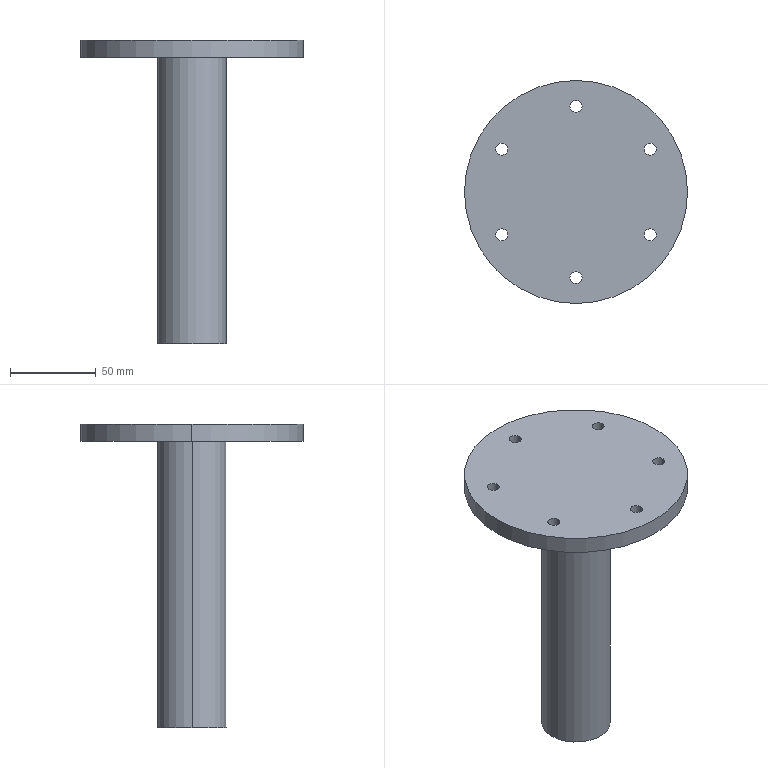Part | SolidWorks | features BaseBody 1 | 1 solid | 22 faces | box 130 x 130 x 177.2 mm | volume 222346 mm3 | cylinder 18 | plane 4 | commonest cylinder face diameters 7 x12 30 x2 40 x2 130 x2
STEP:
#1=CARTESIAN_POINT('',(39.801,25.,167.2));
#2=VERTEX_POINT('',#1);
#3=CARTESIAN_POINT('',(46.801,25.,167.2));
#4=VERTEX_POINT('',#3);
#5=CARTESIAN_POINT('',(43.301,25.,167.2));
#6=DIRECTION('',(0.,0.,1.));
#7=DIRECTION('',(1.,0.,0.));
#8=AXIS2_PLACEMENT_3D('',#5,#6,#7);
#9=CIRCLE('',#8,3.5);
#10=EDGE_CURVE('',#2,#4,#9,.T.);
#11=ORIENTED_EDGE('',*,*,#10,.F.);
#12=CARTESIAN_POINT('',(39.801,25.,177.2));
#13=VERTEX_POINT('',#12);
#14=CARTESIAN_POINT('',(39.801,25.,167.2));
#15=DIRECTION('',(0.,0.,1.));
#16=VECTOR('',#15,1000.);
#17=LINE('',#14,#16);
#18=EDGE_CURVE('',#2,#13,#17,.T.);
#19=ORIENTED_EDGE('',*,*,#18,.T.);
#20=CARTESIAN_POINT('',(46.801,25.,177.2));
#21=VERTEX_POINT('',#20);
#22=CARTESIAN_POINT('',(43.301,25.,177.2));
#23=DIRECTION('',(0.,0.,1.));
#24=DIRECTION('',(1.,0.,0.));
#25=AXIS2_PLACEMENT_3D('',#22,#23,#24);
#26=CIRCLE('',#25,3.5);
#27=EDGE_CURVE('',#13,#21,#26,.T.);
#28=ORIENTED_EDGE('',*,*,#27,.T.);
#29=CARTESIAN_POINT('',(46.801,25.,167.2));
#30=DIRECTION('',(0.,0.,1.));
#31=VECTOR('',#30,1000.);
#32=LINE('',#29,#31);
#33=EDGE_CURVE('',#4,#21,#32,.T.);
#34=ORIENTED_EDGE('',*,*,#33,.F.);
#35=EDGE_LOOP('',(#11,#19,#28,#34));
#36=FACE_OUTER_BOUND('',#35,.T.);
#37=CARTESIAN_POINT('',(43.301,25.,167.2));
#38=DIRECTION('',(0.,0.,1.));
#39=DIRECTION('',(1.,0.,0.));
#40=AXIS2_PLACEMENT_3D('',#37,#38,#39);
#41=CYLINDRICAL_SURFACE('',#40,3.5);
#42=ADVANCED_FACE('',(#36),#41,.F.);
#43=CARTESIAN_POINT('',(39.801,-25.,167.2));
#44=VERTEX_POINT('',#43);
#45=CARTESIAN_POINT('',(46.801,-25.,167.2));
#46=VERTEX_POINT('',#45);
#47=CARTESIAN_POINT('',(43.301,-25.,167.2));
#48=DIRECTION('',(0.,0.,1.));
#49=DIRECTION('',(1.,0.,0.));
#50=AXIS2_PLACEMENT_3D('',#47,#48,#49);
#51=CIRCLE('',#50,3.5);
#52=EDGE_CURVE('',#44,#46,#51,.T.);
#53=ORIENTED_EDGE('',*,*,#52,.F.);
#54=CARTESIAN_POINT('',(39.801,-25.,177.2));
#55=VERTEX_POINT('',#54);
#56=CARTESIAN_POINT('',(39.801,-25.,167.2));
#57=DIRECTION('',(0.,0.,1.));
#58=VECTOR('',#57,1000.);
#59=LINE('',#56,#58);
#60=EDGE_CURVE('',#44,#55,#59,.T.);
#61=ORIENTED_EDGE('',*,*,#60,.T.);
#62=CARTESIAN_POINT('',(46.801,-25.,177.2));
#63=VERTEX_POINT('',#62);
#64=CARTESIAN_POINT('',(43.301,-25.,177.2));
#65=DIRECTION('',(0.,0.,1.));
#66=DIRECTION('',(1.,0.,0.));
#67=AXIS2_PLACEMENT_3D('',#64,#65,#66);
#68=CIRCLE('',#67,3.5);
#69=EDGE_CURVE('',#55,#63,#68,.T.);
#70=ORIENTED_EDGE('',*,*,#69,.T.);
#71=CARTESIAN_POINT('',(46.801,-25.,167.2));
#72=DIRECTION('',(0.,0.,1.));
#73=VECTOR('',#72,1000.);
#74=LINE('',#71,#73);
#75=EDGE_CURVE('',#46,#63,#74,.T.);
#76=ORIENTED_EDGE('',*,*,#75,.F.);
#77=EDGE_LOOP('',(#53,#61,#70,#76));
#78=FACE_OUTER_BOUND('',#77,.T.);
#79=CARTESIAN_POINT('',(43.301,-25.,167.2));
#80=DIRECTION('',(0.,0.,1.));
#81=DIRECTION('',(1.,0.,0.));
#82=AXIS2_PLACEMENT_3D('',#79,#80,#81);
#83=CYLINDRICAL_SURFACE('',#82,3.5);
#84=ADVANCED_FACE('',(#78),#83,.F.);
#85=CARTESIAN_POINT('',(-3.5,-50.,167.2));
#86=VERTEX_POINT('',#85);
#87=CARTESIAN_POINT('',(3.5,-50.,167.2));
#88=VERTEX_POINT('',#87);
#89=CARTESIAN_POINT('',(0.,-50.,167.2));
#90=DIRECTION('',(0.,0.,1.));
#91=DIRECTION('',(1.,0.,0.));
#92=AXIS2_PLACEMENT_3D('',#89,#90,#91);
#93=CIRCLE('',#92,3.5);
#94=EDGE_CURVE('',#86,#88,#93,.T.);
#95=ORIENTED_EDGE('',*,*,#94,.F.);
#96=CARTESIAN_POINT('',(-3.5,-50.,177.2));
#97=VERTEX_POINT('',#96);
#98=CARTESIAN_POINT('',(-3.5,-50.,167.2));
#99=DIRECTION('',(0.,0.,1.));
#100=VECTOR('',#99,1000.);
#101=LINE('',#98,#100);
#102=EDGE_CURVE('',#86,#97,#101,.T.);
#103=ORIENTED_EDGE('',*,*,#102,.T.);
#104=CARTESIAN_POINT('',(3.5,-50.,177.2));
#105=VERTEX_POINT('',#104);
#106=CARTESIAN_POINT('',(0.,-50.,177.2));
#107=DIRECTION('',(0.,0.,1.));
#108=DIRECTION('',(1.,0.,0.));
#109=AXIS2_PLACEMENT_3D('',#106,#107,#108);
#110=CIRCLE('',#109,3.5);
#111=EDGE_CURVE('',#97,#105,#110,.T.);
#112=ORIENTED_EDGE('',*,*,#111,.T.);
#113=CARTESIAN_POINT('',(3.5,-50.,167.2));
#114=DIRECTION('',(0.,0.,1.));
#115=VECTOR('',#114,1000.);
#116=LINE('',#113,#115);
#117=EDGE_CURVE('',#88,#105,#116,.T.);
#118=ORIENTED_EDGE('',*,*,#117,.F.);
#119=EDGE_LOOP('',(#95,#103,#112,#118));
#120=FACE_OUTER_BOUND('',#119,.T.);
#121=CARTESIAN_POINT('',(0.,-50.,167.2));
#122=DIRECTION('',(0.,0.,1.));
#123=DIRECTION('',(1.,0.,0.));
#124=AXIS2_PLACEMENT_3D('',#121,#122,#123);
#125=CYLINDRICAL_SURFACE('',#124,3.5);
#126=ADVANCED_FACE('',(#120),#125,.F.);
#127=CARTESIAN_POINT('',(-46.801,-25.,167.2));
#128=VERTEX_POINT('',#127);
#129=CARTESIAN_POINT('',(-39.801,-25.,167.2));
#130=VERTEX_POINT('',#129);
#131=CARTESIAN_POINT('',(-43.301,-25.,167.2));
#132=DIRECTION('',(0.,0.,1.));
#133=DIRECTION('',(1.,0.,0.));
#134=AXIS2_PLACEMENT_3D('',#131,#132,#133);
#135=CIRCLE('',#134,3.5);
#136=EDGE_CURVE('',#128,#130,#135,.T.);
#137=ORIENTED_EDGE('',*,*,#136,.F.);
#138=CARTESIAN_POINT('',(-46.801,-25.,177.2));
#139=VERTEX_POINT('',#138);
#140=CARTESIAN_POINT('',(-46.801,-25.,167.2));
#141=DIRECTION('',(0.,0.,1.));
#142=VECTOR('',#141,1000.);
#143=LINE('',#140,#142);
#144=EDGE_CURVE('',#128,#139,#143,.T.);
#145=ORIENTED_EDGE('',*,*,#144,.T.);
#146=CARTESIAN_POINT('',(-39.801,-25.,177.2));
#147=VERTEX_POINT('',#146);
#148=CARTESIAN_POINT('',(-43.301,-25.,177.2));
#149=DIRECTION('',(0.,0.,1.));
#150=DIRECTION('',(1.,0.,0.));
#151=AXIS2_PLACEMENT_3D('',#148,#149,#150);
#152=CIRCLE('',#151,3.5);
#153=EDGE_CURVE('',#139,#147,#152,.T.);
#154=ORIENTED_EDGE('',*,*,#153,.T.);
#155=CARTESIAN_POINT('',(-39.801,-25.,167.2));
#156=DIRECTION('',(0.,0.,1.));
#157=VECTOR('',#156,1000.);
#158=LINE('',#155,#157);
#159=EDGE_CURVE('',#130,#147,#158,.T.);
#160=ORIENTED_EDGE('',*,*,#159,.F.);
#161=EDGE_LOOP('',(#137,#145,#154,#160));
#162=FACE_OUTER_BOUND('',#161,.T.);
#163=CARTESIAN_POINT('',(-43.301,-25.,167.2));
#164=DIRECTION('',(0.,0.,1.));
#165=DIRECTION('',(1.,0.,0.));
#166=AXIS2_PLACEMENT_3D('',#163,#164,#165);
#167=CYLINDRICAL_SURFACE('',#166,3.5);
#168=ADVANCED_FACE('',(#162),#167,.F.);
#169=CARTESIAN_POINT('',(-46.801,25.,167.2));
#170=VERTEX_POINT('',#169);
#171=CARTESIAN_POINT('',(-39.801,25.,167.2));
#172=VERTEX_POINT('',#171);
#173=CARTESIAN_POINT('',(-43.301,25.,167.2));
#174=DIRECTION('',(0.,0.,1.));
#175=DIRECTION('',(1.,0.,0.));
#176=AXIS2_PLACEMENT_3D('',#173,#174,#175);
#177=CIRCLE('',#176,3.5);
#178=EDGE_CURVE('',#170,#172,#177,.T.);
#179=ORIENTED_EDGE('',*,*,#178,.F.);
#180=CARTESIAN_POINT('',(-46.801,25.,177.2));
#181=VERTEX_POINT('',#180);
#182=CARTESIAN_POINT('',(-46.801,25.,167.2));
#183=DIRECTION('',(0.,0.,1.));
#184=VECTOR('',#183,1000.);
#185=LINE('',#182,#184);
#186=EDGE_CURVE('',#170,#181,#185,.T.);
#187=ORIENTED_EDGE('',*,*,#186,.T.);
#188=CARTESIAN_POINT('',(-39.801,25.,177.2));
#189=VERTEX_POINT('',#188);
#190=CARTESIAN_POINT('',(-43.301,25.,177.2));
#191=DIRECTION('',(0.,0.,1.));
#192=DIRECTION('',(1.,0.,0.));
#193=AXIS2_PLACEMENT_3D('',#190,#191,#192);
#194=CIRCLE('',#193,3.5);
#195=EDGE_CURVE('',#181,#189,#194,.T.);
#196=ORIENTED_EDGE('',*,*,#195,.T.);
#197=CARTESIAN_POINT('',(-39.801,25.,167.2));
#198=DIRECTION('',(0.,0.,1.));
#199=VECTOR('',#198,1000.);
#200=LINE('',#197,#199);
#201=EDGE_CURVE('',#172,#189,#200,.T.);
#202=ORIENTED_EDGE('',*,*,#201,.F.);
#203=EDGE_LOOP('',(#179,#187,#196,#202));
#204=FACE_OUTER_BOUND('',#203,.T.);
#205=CARTESIAN_POINT('',(-43.301,25.,167.2));
#206=DIRECTION('',(0.,0.,1.));
#207=DIRECTION('',(1.,0.,0.));
#208=AXIS2_PLACEMENT_3D('',#205,#206,#207);
#209=CYLINDRICAL_SURFACE('',#208,3.5);
#210=ADVANCED_FACE('',(#204),#209,.F.);
#211=CARTESIAN_POINT('',(-3.5,50.,167.2));
#212=VERTEX_POINT('',#211);
#213=CARTESIAN_POINT('',(3.5,50.,167.2));
#214=VERTEX_POINT('',#213);
#215=CARTESIAN_POINT('',(0.,50.,167.2));
#216=DIRECTION('',(0.,0.,1.));
#217=DIRECTION('',(1.,0.,0.));
#218=AXIS2_PLACEMENT_3D('',#215,#216,#217);
#219=CIRCLE('',#218,3.5);
#220=EDGE_CURVE('',#212,#214,#219,.T.);
#221=ORIENTED_EDGE('',*,*,#220,.F.);
#222=CARTESIAN_POINT('',(-3.5,50.,177.2));
#223=VERTEX_POINT('',#222);
#224=CARTESIAN_POINT('',(-3.5,50.,167.2));
#225=DIRECTION('',(0.,0.,1.));
#226=VECTOR('',#225,1000.);
#227=LINE('',#224,#226);
#228=EDGE_CURVE('',#212,#223,#227,.T.);
#229=ORIENTED_EDGE('',*,*,#228,.T.);
#230=CARTESIAN_POINT('',(3.5,50.,177.2));
#231=VERTEX_POINT('',#230);
#232=CARTESIAN_POINT('',(0.,50.,177.2));
#233=DIRECTION('',(0.,0.,1.));
#234=DIRECTION('',(1.,0.,0.));
#235=AXIS2_PLACEMENT_3D('',#232,#233,#234);
#236=CIRCLE('',#235,3.5);
#237=EDGE_CURVE('',#223,#231,#236,.T.);
#238=ORIENTED_EDGE('',*,*,#237,.T.);
#239=CARTESIAN_POINT('',(3.5,50.,167.2));
#240=DIRECTION('',(0.,0.,1.));
#241=VECTOR('',#240,1000.);
#242=LINE('',#239,#241);
#243=EDGE_CURVE('',#214,#231,#242,.T.);
#244=ORIENTED_EDGE('',*,*,#243,.F.);
#245=EDGE_LOOP('',(#221,#229,#238,#244));
#246=FACE_OUTER_BOUND('',#245,.T.);
#247=CARTESIAN_POINT('',(0.,50.,167.2));
#248=DIRECTION('',(0.,0.,1.));
#249=DIRECTION('',(1.,0.,0.));
#250=AXIS2_PLACEMENT_3D('',#247,#248,#249);
#251=CYLINDRICAL_SURFACE('',#250,3.5);
#252=ADVANCED_FACE('',(#246),#251,.F.);
#253=CARTESIAN_POINT('',(65.,0.,167.2));
#254=VERTEX_POINT('',#253);
#255=CARTESIAN_POINT('',(-65.,0.,167.2));
#256=VERTEX_POINT('',#255);
#257=CARTESIAN_POINT('',(0.,0.,167.2));
#258=DIRECTION('',(0.,0.,1.));
#259=DIRECTION('',(1.,0.,0.));
#260=AXIS2_PLACEMENT_3D('',#257,#258,#259);
#261=CIRCLE('',#260,65.);
#262=EDGE_CURVE('',#254,#256,#261,.T.);
#263=ORIENTED_EDGE('',*,*,#262,.T.);
#264=CARTESIAN_POINT('',(-65.,0.,177.2));
#265=VERTEX_POINT('',#264);
#266=CARTESIAN_POINT('',(-65.,0.,167.2));
#267=DIRECTION('',(0.,0.,1.));
#268=VECTOR('',#267,1000.);
#269=LINE('',#266,#268);
#270=EDGE_CURVE('',#256,#265,#269,.T.);
#271=ORIENTED_EDGE('',*,*,#270,.T.);
#272=CARTESIAN_POINT('',(65.,0.,177.2));
#273=VERTEX_POINT('',#272);
#274=CARTESIAN_POINT('',(0.,0.,177.2));
#275=DIRECTION('',(0.,0.,-1.));
#276=DIRECTION('',(1.,0.,0.));
#277=AXIS2_PLACEMENT_3D('',#274,#275,#276);
#278=CIRCLE('',#277,65.);
#279=EDGE_CURVE('',#265,#273,#278,.T.);
#280=ORIENTED_EDGE('',*,*,#279,.T.);
#281=CARTESIAN_POINT('',(65.,0.,167.2));
#282=DIRECTION('',(0.,0.,1.));
#283=VECTOR('',#282,1000.);
#284=LINE('',#281,#283);
#285=EDGE_CURVE('',#254,#273,#284,.T.);
#286=ORIENTED_EDGE('',*,*,#285,.F.);
#287=EDGE_LOOP('',(#263,#271,#280,#286));
#288=FACE_OUTER_BOUND('',#287,.T.);
#289=CARTESIAN_POINT('',(0.,0.,167.2));
#290=DIRECTION('',(0.,0.,1.));
#291=DIRECTION('',(1.,0.,0.));
#292=AXIS2_PLACEMENT_3D('',#289,#290,#291);
#293=CYLINDRICAL_SURFACE('',#292,65.);
#294=ADVANCED_FACE('',(#288),#293,.T.);
#295=CARTESIAN_POINT('',(20.,0.,167.2));
#296=VERTEX_POINT('',#295);
#297=CARTESIAN_POINT('',(-20.,0.,167.2));
#298=VERTEX_POINT('',#297);
#299=CARTESIAN_POINT('',(0.,0.,167.2));
#300=DIRECTION('',(0.,0.,1.));
#301=DIRECTION('',(-1.,0.,0.));
#302=AXIS2_PLACEMENT_3D('',#299,#300,#301);
#303=CIRCLE('',#302,20.);
#304=EDGE_CURVE('',#296,#298,#303,.T.);
#305=ORIENTED_EDGE('',*,*,#304,.F.);
#306=CARTESIAN_POINT('',(20.,0.,0.));
#307=VERTEX_POINT('',#306);
#308=CARTESIAN_POINT('',(20.,0.,233.769));
#309=DIRECTION('',(0.,0.,-1.));
#310=VECTOR('',#309,1000.);
#311=LINE('',#308,#310);
#312=EDGE_CURVE('',#296,#307,#311,.T.);
#313=ORIENTED_EDGE('',*,*,#312,.T.);
#314=CARTESIAN_POINT('',(-20.,0.,0.));
#315=VERTEX_POINT('',#314);
#316=CARTESIAN_POINT('',(0.,0.,0.));
#317=DIRECTION('',(0.,0.,1.));
#318=DIRECTION('',(-1.,0.,0.));
#319=AXIS2_PLACEMENT_3D('',#316,#317,#318);
#320=CIRCLE('',#319,20.);
#321=EDGE_CURVE('',#307,#315,#320,.T.);
#322=ORIENTED_EDGE('',*,*,#321,.T.);
#323=CARTESIAN_POINT('',(-20.,0.,233.769));
#324=DIRECTION('',(0.,0.,-1.));
#325=VECTOR('',#324,1000.);
#326=LINE('',#323,#325);
#327=EDGE_CURVE('',#298,#315,#326,.T.);
#328=ORIENTED_EDGE('',*,*,#327,.F.);
#329=EDGE_LOOP('',(#305,#313,#322,#328));
#330=FACE_OUTER_BOUND('',#329,.T.);
#331=CARTESIAN_POINT('',(0.,0.,233.769));
#332=DIRECTION('',(0.,0.,-1.));
#333=DIRECTION('',(-1.,0.,0.));
#334=AXIS2_PLACEMENT_3D('',#331,#332,#333);
#335=CYLINDRICAL_SURFACE('',#334,20.);
#336=ADVANCED_FACE('',(#330),#335,.T.);
#337=CARTESIAN_POINT('',(15.,0.,167.2));
#338=VERTEX_POINT('',#337);
#339=CARTESIAN_POINT('',(-15.,0.,167.2));
#340=VERTEX_POINT('',#339);
#341=CARTESIAN_POINT('',(0.,0.,167.2));
#342=DIRECTION('',(0.,0.,-1.));
#343=DIRECTION('',(-1.,0.,0.));
#344=AXIS2_PLACEMENT_3D('',#341,#342,#343);
#345=CIRCLE('',#344,15.);
#346=EDGE_CURVE('',#338,#340,#345,.T.);
#347=ORIENTED_EDGE('',*,*,#346,.F.);
#348=CARTESIAN_POINT('',(15.,0.,0.));
#349=VERTEX_POINT('',#348);
#350=CARTESIAN_POINT('',(15.,0.,233.769));
#351=DIRECTION('',(0.,0.,-1.));
#352=VECTOR('',#351,1000.);
#353=LINE('',#350,#352);
#354=EDGE_CURVE('',#338,#349,#353,.T.);
#355=ORIENTED_EDGE('',*,*,#354,.T.);
#356=CARTESIAN_POINT('',(-15.,0.,0.));
#357=VERTEX_POINT('',#356);
#358=CARTESIAN_POINT('',(0.,0.,0.));
#359=DIRECTION('',(0.,0.,-1.));
#360=DIRECTION('',(-1.,0.,0.));
#361=AXIS2_PLACEMENT_3D('',#358,#359,#360);
#362=CIRCLE('',#361,15.);
#363=EDGE_CURVE('',#349,#357,#362,.T.);
#364=ORIENTED_EDGE('',*,*,#363,.T.);
#365=CARTESIAN_POINT('',(-15.,0.,233.769));
#366=DIRECTION('',(0.,0.,-1.));
#367=VECTOR('',#366,1000.);
#368=LINE('',#365,#367);
#369=EDGE_CURVE('',#340,#357,#368,.T.);
#370=ORIENTED_EDGE('',*,*,#369,.F.);
#371=EDGE_LOOP('',(#347,#355,#364,#370));
#372=FACE_OUTER_BOUND('',#371,.T.);
#373=CARTESIAN_POINT('',(0.,0.,233.769));
#374=DIRECTION('',(0.,0.,-1.));
#375=DIRECTION('',(-1.,0.,0.));
#376=AXIS2_PLACEMENT_3D('',#373,#374,#375);
#377=CYLINDRICAL_SURFACE('',#376,15.);
#378=ADVANCED_FACE('',(#372),#377,.F.);
#379=CARTESIAN_POINT('',(43.301,25.,177.2));
#380=DIRECTION('',(0.,0.,1.));
#381=DIRECTION('',(1.,0.,0.));
#382=AXIS2_PLACEMENT_3D('',#379,#380,#381);
#383=CIRCLE('',#382,3.5);
#384=EDGE_CURVE('',#21,#13,#383,.T.);
#385=ORIENTED_EDGE('',*,*,#384,.F.);
#386=ORIENTED_EDGE('',*,*,#27,.F.);
#387=EDGE_LOOP('',(#385,#386));
#388=FACE_BOUND('',#387,.T.);
#389=CARTESIAN_POINT('',(43.301,-25.,177.2));
#390=DIRECTION('',(0.,0.,1.));
#391=DIRECTION('',(1.,0.,0.));
#392=AXIS2_PLACEMENT_3D('',#389,#390,#391);
#393=CIRCLE('',#392,3.5);
#394=EDGE_CURVE('',#63,#55,#393,.T.);
#395=ORIENTED_EDGE('',*,*,#394,.F.);
#396=ORIENTED_EDGE('',*,*,#69,.F.);
#397=EDGE_LOOP('',(#395,#396));
#398=FACE_BOUND('',#397,.T.);
#399=CARTESIAN_POINT('',(0.,-50.,177.2));
#400=DIRECTION('',(0.,0.,1.));
#401=DIRECTION('',(1.,0.,0.));
#402=AXIS2_PLACEMENT_3D('',#399,#400,#401);
#403=CIRCLE('',#402,3.5);
#404=EDGE_CURVE('',#105,#97,#403,.T.);
#405=ORIENTED_EDGE('',*,*,#404,.F.);
#406=ORIENTED_EDGE('',*,*,#111,.F.);
#407=EDGE_LOOP('',(#405,#406));
#408=FACE_BOUND('',#407,.T.);
#409=CARTESIAN_POINT('',(-43.301,-25.,177.2));
#410=DIRECTION('',(0.,0.,1.));
#411=DIRECTION('',(1.,0.,0.));
#412=AXIS2_PLACEMENT_3D('',#409,#410,#411);
#413=CIRCLE('',#412,3.5);
#414=EDGE_CURVE('',#147,#139,#413,.T.);
#415=ORIENTED_EDGE('',*,*,#414,.F.);
#416=ORIENTED_EDGE('',*,*,#153,.F.);
#417=EDGE_LOOP('',(#415,#416));
#418=FACE_BOUND('',#417,.T.);
#419=CARTESIAN_POINT('',(-43.301,25.,177.2));
#420=DIRECTION('',(0.,0.,1.));
#421=DIRECTION('',(1.,0.,0.));
#422=AXIS2_PLACEMENT_3D('',#419,#420,#421);
#423=CIRCLE('',#422,3.5);
#424=EDGE_CURVE('',#189,#181,#423,.T.);
#425=ORIENTED_EDGE('',*,*,#424,.F.);
#426=ORIENTED_EDGE('',*,*,#195,.F.);
#427=EDGE_LOOP('',(#425,#426));
#428=FACE_BOUND('',#427,.T.);
#429=CARTESIAN_POINT('',(0.,50.,177.2));
#430=DIRECTION('',(0.,0.,1.));
#431=DIRECTION('',(1.,0.,0.));
#432=AXIS2_PLACEMENT_3D('',#429,#430,#431);
#433=CIRCLE('',#432,3.5);
#434=EDGE_CURVE('',#231,#223,#433,.T.);
#435=ORIENTED_EDGE('',*,*,#434,.F.);
#436=ORIENTED_EDGE('',*,*,#237,.F.);
#437=EDGE_LOOP('',(#435,#436));
#438=FACE_BOUND('',#437,.T.);
#439=CARTESIAN_POINT('',(0.,0.,177.2));
#440=DIRECTION('',(0.,0.,-1.));
#441=DIRECTION('',(1.,0.,0.));
#442=AXIS2_PLACEMENT_3D('',#439,#440,#441);
#443=CIRCLE('',#442,65.);
#444=EDGE_CURVE('',#273,#265,#443,.T.);
#445=ORIENTED_EDGE('',*,*,#444,.F.);
#446=ORIENTED_EDGE('',*,*,#279,.F.);
#447=EDGE_LOOP('',(#445,#446));
#448=FACE_OUTER_BOUND('',#447,.T.);
#449=CARTESIAN_POINT('',(431.187,336.743,177.2));
#450=DIRECTION('',(0.,0.,-1.));
#451=DIRECTION('',(0.,1.,0.));
#452=AXIS2_PLACEMENT_3D('',#449,#450,#451);
#453=PLANE('',#452);
#454=ADVANCED_FACE('',(#388,#398,#408,#418,#428,#438,#448),#453,.F.);
#455=ORIENTED_EDGE('',*,*,#18,.F.);
#456=CARTESIAN_POINT('',(43.301,25.,167.2));
#457=DIRECTION('',(0.,0.,1.));
#458=DIRECTION('',(1.,0.,0.));
#459=AXIS2_PLACEMENT_3D('',#456,#457,#458);
#460=CIRCLE('',#459,3.5);
#461=EDGE_CURVE('',#4,#2,#460,.T.);
#462=ORIENTED_EDGE('',*,*,#461,.F.);
#463=ORIENTED_EDGE('',*,*,#33,.T.);
#464=ORIENTED_EDGE('',*,*,#384,.T.);
#465=EDGE_LOOP('',(#455,#462,#463,#464));
#466=FACE_OUTER_BOUND('',#465,.T.);
#467=CARTESIAN_POINT('',(43.301,25.,167.2));
#468=DIRECTION('',(0.,0.,1.));
#469=DIRECTION('',(1.,0.,0.));
#470=AXIS2_PLACEMENT_3D('',#467,#468,#469);
#471=CYLINDRICAL_SURFACE('',#470,3.5);
#472=ADVANCED_FACE('',(#466),#471,.F.);
#473=ORIENTED_EDGE('',*,*,#60,.F.);
#474=CARTESIAN_POINT('',(43.301,-25.,167.2));
#475=DIRECTION('',(0.,0.,1.));
#476=DIRECTION('',(1.,0.,0.));
#477=AXIS2_PLACEMENT_3D('',#474,#475,#476);
#478=CIRCLE('',#477,3.5);
#479=EDGE_CURVE('',#46,#44,#478,.T.);
#480=ORIENTED_EDGE('',*,*,#479,.F.);
#481=ORIENTED_EDGE('',*,*,#75,.T.);
#482=ORIENTED_EDGE('',*,*,#394,.T.);
#483=EDGE_LOOP('',(#473,#480,#481,#482));
#484=FACE_OUTER_BOUND('',#483,.T.);
#485=CARTESIAN_POINT('',(43.301,-25.,167.2));
#486=DIRECTION('',(0.,0.,1.));
#487=DIRECTION('',(1.,0.,0.));
#488=AXIS2_PLACEMENT_3D('',#485,#486,#487);
#489=CYLINDRICAL_SURFACE('',#488,3.5);
#490=ADVANCED_FACE('',(#484),#489,.F.);
#491=ORIENTED_EDGE('',*,*,#102,.F.);
#492=CARTESIAN_POINT('',(0.,-50.,167.2));
#493=DIRECTION('',(0.,0.,1.));
#494=DIRECTION('',(1.,0.,0.));
#495=AXIS2_PLACEMENT_3D('',#492,#493,#494);
#496=CIRCLE('',#495,3.5);
#497=EDGE_CURVE('',#88,#86,#496,.T.);
#498=ORIENTED_EDGE('',*,*,#497,.F.);
#499=ORIENTED_EDGE('',*,*,#117,.T.);
#500=ORIENTED_EDGE('',*,*,#404,.T.);
#501=EDGE_LOOP('',(#491,#498,#499,#500));
#502=FACE_OUTER_BOUND('',#501,.T.);
#503=CARTESIAN_POINT('',(0.,-50.,167.2));
#504=DIRECTION('',(0.,0.,1.));
#505=DIRECTION('',(1.,0.,0.));
#506=AXIS2_PLACEMENT_3D('',#503,#504,#505);
#507=CYLINDRICAL_SURFACE('',#506,3.5);
#508=ADVANCED_FACE('',(#502),#507,.F.);
#509=ORIENTED_EDGE('',*,*,#144,.F.);
#510=CARTESIAN_POINT('',(-43.301,-25.,167.2));
#511=DIRECTION('',(0.,0.,1.));
#512=DIRECTION('',(1.,0.,0.));
#513=AXIS2_PLACEMENT_3D('',#510,#511,#512);
#514=CIRCLE('',#513,3.5);
#515=EDGE_CURVE('',#130,#128,#514,.T.);
#516=ORIENTED_EDGE('',*,*,#515,.F.);
#517=ORIENTED_EDGE('',*,*,#159,.T.);
#518=ORIENTED_EDGE('',*,*,#414,.T.);
#519=EDGE_LOOP('',(#509,#516,#517,#518));
#520=FACE_OUTER_BOUND('',#519,.T.);
#521=CARTESIAN_POINT('',(-43.301,-25.,167.2));
#522=DIRECTION('',(0.,0.,1.));
#523=DIRECTION('',(1.,0.,0.));
#524=AXIS2_PLACEMENT_3D('',#521,#522,#523);
#525=CYLINDRICAL_SURFACE('',#524,3.5);
#526=ADVANCED_FACE('',(#520),#525,.F.);
#527=ORIENTED_EDGE('',*,*,#186,.F.);
#528=CARTESIAN_POINT('',(-43.301,25.,167.2));
#529=DIRECTION('',(0.,0.,1.));
#530=DIRECTION('',(1.,0.,0.));
#531=AXIS2_PLACEMENT_3D('',#528,#529,#530);
#532=CIRCLE('',#531,3.5);
#533=EDGE_CURVE('',#172,#170,#532,.T.);
#534=ORIENTED_EDGE('',*,*,#533,.F.);
#535=ORIENTED_EDGE('',*,*,#201,.T.);
#536=ORIENTED_EDGE('',*,*,#424,.T.);
#537=EDGE_LOOP('',(#527,#534,#535,#536));
#538=FACE_OUTER_BOUND('',#537,.T.);
#539=CARTESIAN_POINT('',(-43.301,25.,167.2));
#540=DIRECTION('',(0.,0.,1.));
#541=DIRECTION('',(1.,0.,0.));
#542=AXIS2_PLACEMENT_3D('',#539,#540,#541);
#543=CYLINDRICAL_SURFACE('',#542,3.5);
#544=ADVANCED_FACE('',(#538),#543,.F.);
#545=ORIENTED_EDGE('',*,*,#228,.F.);
#546=CARTESIAN_POINT('',(0.,50.,167.2));
#547=DIRECTION('',(0.,0.,1.));
#548=DIRECTION('',(1.,0.,0.));
#549=AXIS2_PLACEMENT_3D('',#546,#547,#548);
#550=CIRCLE('',#549,3.5);
#551=EDGE_CURVE('',#214,#212,#550,.T.);
#552=ORIENTED_EDGE('',*,*,#551,.F.);
#553=ORIENTED_EDGE('',*,*,#243,.T.);
#554=ORIENTED_EDGE('',*,*,#434,.T.);
#555=EDGE_LOOP('',(#545,#552,#553,#554));
#556=FACE_OUTER_BOUND('',#555,.T.);
#557=CARTESIAN_POINT('',(0.,50.,167.2));
#558=DIRECTION('',(0.,0.,1.));
#559=DIRECTION('',(1.,0.,0.));
#560=AXIS2_PLACEMENT_3D('',#557,#558,#559);
#561=CYLINDRICAL_SURFACE('',#560,3.5);
#562=ADVANCED_FACE('',(#556),#561,.F.);
#563=ORIENTED_EDGE('',*,*,#270,.F.);
#564=CARTESIAN_POINT('',(0.,0.,167.2));
#565=DIRECTION('',(0.,0.,1.));
#566=DIRECTION('',(1.,0.,0.));
#567=AXIS2_PLACEMENT_3D('',#564,#565,#566);
#568=CIRCLE('',#567,65.);
#569=EDGE_CURVE('',#256,#254,#568,.T.);
#570=ORIENTED_EDGE('',*,*,#569,.T.);
#571=ORIENTED_EDGE('',*,*,#285,.T.);
#572=ORIENTED_EDGE('',*,*,#444,.T.);
#573=EDGE_LOOP('',(#563,#570,#571,#572));
#574=FACE_OUTER_BOUND('',#573,.T.);
#575=CARTESIAN_POINT('',(0.,0.,167.2));
#576=DIRECTION('',(0.,0.,1.));
#577=DIRECTION('',(1.,0.,0.));
#578=AXIS2_PLACEMENT_3D('',#575,#576,#577);
#579=CYLINDRICAL_SURFACE('',#578,65.);
#580=ADVANCED_FACE('',(#574),#579,.T.);
#581=ORIENTED_EDGE('',*,*,#461,.T.);
#582=ORIENTED_EDGE('',*,*,#10,.T.);
#583=EDGE_LOOP('',(#581,#582));
#584=FACE_BOUND('',#583,.T.);
#585=ORIENTED_EDGE('',*,*,#497,.T.);
#586=ORIENTED_EDGE('',*,*,#94,.T.);
#587=EDGE_LOOP('',(#585,#586));
#588=FACE_BOUND('',#587,.T.);
#589=ORIENTED_EDGE('',*,*,#533,.T.);
#590=ORIENTED_EDGE('',*,*,#178,.T.);
#591=EDGE_LOOP('',(#589,#590));
#592=FACE_BOUND('',#591,.T.);
#593=ORIENTED_EDGE('',*,*,#262,.F.);
#594=ORIENTED_EDGE('',*,*,#569,.F.);
#595=EDGE_LOOP('',(#593,#594));
#596=FACE_OUTER_BOUND('',#595,.T.);
#597=ORIENTED_EDGE('',*,*,#551,.T.);
#598=ORIENTED_EDGE('',*,*,#220,.T.);
#599=EDGE_LOOP('',(#597,#598));
#600=FACE_BOUND('',#599,.T.);
#601=ORIENTED_EDGE('',*,*,#515,.T.);
#602=ORIENTED_EDGE('',*,*,#136,.T.);
#603=EDGE_LOOP('',(#601,#602));
#604=FACE_BOUND('',#603,.T.);
#605=ORIENTED_EDGE('',*,*,#479,.T.);
#606=ORIENTED_EDGE('',*,*,#52,.T.);
#607=EDGE_LOOP('',(#605,#606));
#608=FACE_BOUND('',#607,.T.);
#609=CARTESIAN_POINT('',(0.,0.,167.2));
#610=DIRECTION('',(0.,0.,1.));
#611=DIRECTION('',(-1.,0.,0.));
#612=AXIS2_PLACEMENT_3D('',#609,#610,#611);
#613=CIRCLE('',#612,20.);
#614=EDGE_CURVE('',#298,#296,#613,.T.);
#615=ORIENTED_EDGE('',*,*,#614,.T.);
#616=ORIENTED_EDGE('',*,*,#304,.T.);
#617=EDGE_LOOP('',(#615,#616));
#618=FACE_BOUND('',#617,.T.);
#619=CARTESIAN_POINT('',(0.,0.,167.2));
#620=DIRECTION('',(0.,0.,-1.));
#621=DIRECTION('',(-1.,0.,0.));
#622=AXIS2_PLACEMENT_3D('',#619,#620,#621);
#623=PLANE('',#622);
#624=ADVANCED_FACE('',(#584,#588,#592,#596,#600,#604,#608,#618),#623,.T.);
#625=ORIENTED_EDGE('',*,*,#312,.F.);
#626=ORIENTED_EDGE('',*,*,#614,.F.);
#627=ORIENTED_EDGE('',*,*,#327,.T.);
#628=CARTESIAN_POINT('',(0.,0.,0.));
#629=DIRECTION('',(0.,0.,1.));
#630=DIRECTION('',(-1.,0.,0.));
#631=AXIS2_PLACEMENT_3D('',#628,#629,#630);
#632=CIRCLE('',#631,20.);
#633=EDGE_CURVE('',#315,#307,#632,.T.);
#634=ORIENTED_EDGE('',*,*,#633,.T.);
#635=EDGE_LOOP('',(#625,#626,#627,#634));
#636=FACE_OUTER_BOUND('',#635,.T.);
#637=CARTESIAN_POINT('',(0.,0.,233.769));
#638=DIRECTION('',(0.,0.,-1.));
#639=DIRECTION('',(-1.,0.,0.));
#640=AXIS2_PLACEMENT_3D('',#637,#638,#639);
#641=CYLINDRICAL_SURFACE('',#640,20.);
#642=ADVANCED_FACE('',(#636),#641,.T.);
#643=CARTESIAN_POINT('',(0.,0.,0.));
#644=DIRECTION('',(0.,0.,-1.));
#645=DIRECTION('',(-1.,0.,0.));
#646=AXIS2_PLACEMENT_3D('',#643,#644,#645);
#647=CIRCLE('',#646,15.);
#648=EDGE_CURVE('',#357,#349,#647,.T.);
#649=ORIENTED_EDGE('',*,*,#648,.F.);
#650=ORIENTED_EDGE('',*,*,#363,.F.);
#651=EDGE_LOOP('',(#649,#650));
#652=FACE_BOUND('',#651,.T.);
#653=ORIENTED_EDGE('',*,*,#633,.F.);
#654=ORIENTED_EDGE('',*,*,#321,.F.);
#655=EDGE_LOOP('',(#653,#654));
#656=FACE_OUTER_BOUND('',#655,.T.);
#657=CARTESIAN_POINT('',(0.,0.,0.));
#658=DIRECTION('',(0.,0.,1.));
#659=DIRECTION('',(1.,0.,0.));
#660=AXIS2_PLACEMENT_3D('',#657,#658,#659);
#661=PLANE('',#660);
#662=ADVANCED_FACE('',(#652,#656),#661,.F.);
#663=ORIENTED_EDGE('',*,*,#354,.F.);
#664=CARTESIAN_POINT('',(0.,0.,167.2));
#665=DIRECTION('',(0.,0.,-1.));
#666=DIRECTION('',(-1.,0.,0.));
#667=AXIS2_PLACEMENT_3D('',#664,#665,#666);
#668=CIRCLE('',#667,15.);
#669=EDGE_CURVE('',#340,#338,#668,.T.);
#670=ORIENTED_EDGE('',*,*,#669,.F.);
#671=ORIENTED_EDGE('',*,*,#369,.T.);
#672=ORIENTED_EDGE('',*,*,#648,.T.);
#673=EDGE_LOOP('',(#663,#670,#671,#672));
#674=FACE_OUTER_BOUND('',#673,.T.);
#675=CARTESIAN_POINT('',(0.,0.,233.769));
#676=DIRECTION('',(0.,0.,-1.));
#677=DIRECTION('',(-1.,0.,0.));
#678=AXIS2_PLACEMENT_3D('',#675,#676,#677);
#679=CYLINDRICAL_SURFACE('',#678,15.);
#680=ADVANCED_FACE('',(#674),#679,.F.);
#681=ORIENTED_EDGE('',*,*,#669,.T.);
#682=ORIENTED_EDGE('',*,*,#346,.T.);
#683=EDGE_LOOP('',(#681,#682));
#684=FACE_OUTER_BOUND('',#683,.T.);
#685=CARTESIAN_POINT('',(0.,0.,167.2));
#686=DIRECTION('',(0.,0.,-1.));
#687=DIRECTION('',(-1.,0.,0.));
#688=AXIS2_PLACEMENT_3D('',#685,#686,#687);
#689=PLANE('',#688);
#690=ADVANCED_FACE('',(#684),#689,.T.);
#691=CLOSED_SHELL('',(#42,#84,#126,#168,#210,#252,#294,#336,#378,#454,#472,#490,#508,#526,#544,#562,#580,#624,#642,#662,#680,#690));
#692=MANIFOLD_SOLID_BREP('',#691);
#693=CARTESIAN_POINT('',(0.,0.,0.));
#694=DIRECTION('',(0.,0.,1.));
#695=DIRECTION('',(1.,0.,0.));
#696=AXIS2_PLACEMENT_3D('',#693,#694,#695);
#697=(LENGTH_UNIT()NAMED_UNIT(*)SI_UNIT(.MILLI.,.METRE.));
#698=UNCERTAINTY_MEASURE_WITH_UNIT(LENGTH_MEASURE(0.00001),#697,'','');
#699=(NAMED_UNIT(*)PLANE_ANGLE_UNIT()SI_UNIT($,.RADIAN.));
#700=(NAMED_UNIT(*)SI_UNIT($,.STERADIAN.)SOLID_ANGLE_UNIT());
#701=(GEOMETRIC_REPRESENTATION_CONTEXT(3)GLOBAL_UNCERTAINTY_ASSIGNED_CONTEXT((#698))GLOBAL_UNIT_ASSIGNED_CONTEXT((#697,#699,#700))REPRESENTATION_CONTEXT('',''));
#702=ADVANCED_BREP_SHAPE_REPRESENTATION('',(#692,#696),#701);